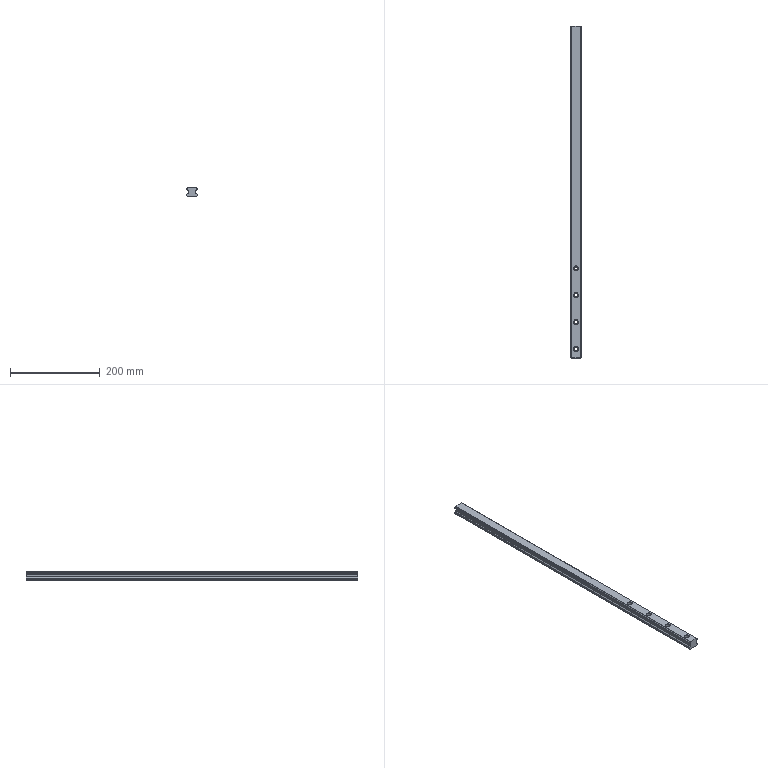Part | 1 solid | 58 faces | box 23 x 740 x 20 mm | volume 297634 mm3 | cylinder 38 | plane 20 | commonest cylinder face diameters 7 x8 11 x8 0.6 x4 0.594 x2 0.973 x2 0.985 x2